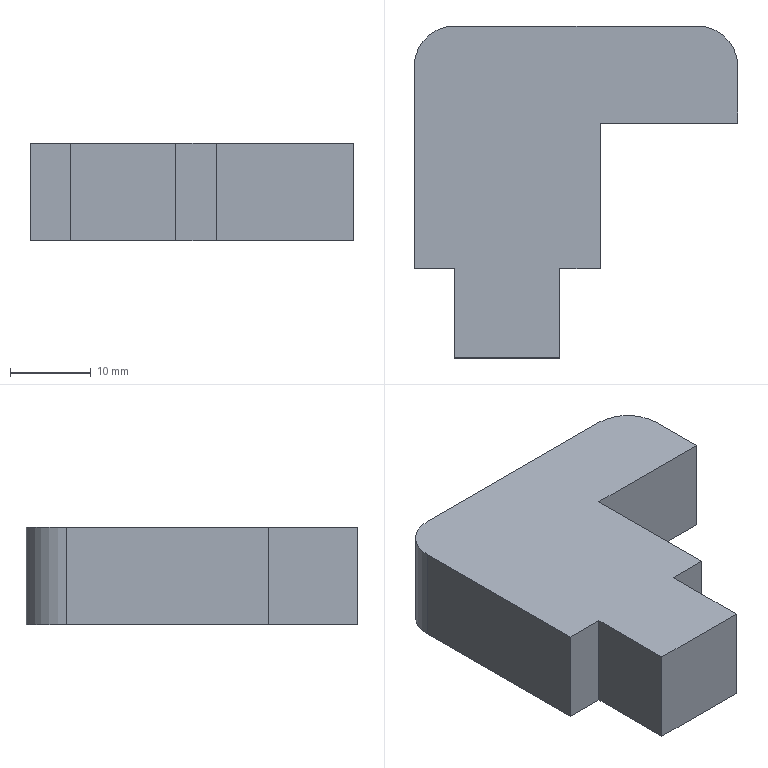Part | SolidWorks | features Fillet 1, FlatPattern 1, SMBaseFlange 1, SheetMetal 1 | 1 solid | 14 faces | box 40 x 41 x 12 mm | volume 12315 mm3 | plane 12 | cylinder 2 | commonest cylinder face diameters 10 x2
STEP:
#1=CARTESIAN_POINT('',(-40.,-14.,0.));
#2=VERTEX_POINT('',#1);
#3=CARTESIAN_POINT('',(-35.,-14.,0.));
#4=VERTEX_POINT('',#3);
#5=CARTESIAN_POINT('',(-35.,-14.,0.));
#6=DIRECTION('',(1.,0.,0.));
#7=VECTOR('',#6,1000.);
#8=LINE('',#5,#7);
#9=EDGE_CURVE('',#2,#4,#8,.T.);
#10=ORIENTED_EDGE('',*,*,#9,.F.);
#11=CARTESIAN_POINT('',(-40.,-14.,-12.));
#12=VERTEX_POINT('',#11);
#13=CARTESIAN_POINT('',(-40.,-14.,-12.));
#14=DIRECTION('',(0.,0.,1.));
#15=VECTOR('',#14,1000.);
#16=LINE('',#13,#15);
#17=EDGE_CURVE('',#12,#2,#16,.T.);
#18=ORIENTED_EDGE('',*,*,#17,.F.);
#19=CARTESIAN_POINT('',(-35.,-14.,-12.));
#20=VERTEX_POINT('',#19);
#21=CARTESIAN_POINT('',(-35.,-14.,-12.));
#22=DIRECTION('',(1.,0.,0.));
#23=VECTOR('',#22,1000.);
#24=LINE('',#21,#23);
#25=EDGE_CURVE('',#12,#20,#24,.T.);
#26=ORIENTED_EDGE('',*,*,#25,.T.);
#27=CARTESIAN_POINT('',(-35.,-14.,-12.));
#28=DIRECTION('',(0.,0.,1.));
#29=VECTOR('',#28,1000.);
#30=LINE('',#27,#29);
#31=EDGE_CURVE('',#20,#4,#30,.T.);
#32=ORIENTED_EDGE('',*,*,#31,.T.);
#33=EDGE_LOOP('',(#10,#18,#26,#32));
#34=FACE_OUTER_BOUND('',#33,.T.);
#35=CARTESIAN_POINT('',(-35.,-14.,-12.));
#36=DIRECTION('',(0.,-1.,0.));
#37=DIRECTION('',(1.,0.,0.));
#38=AXIS2_PLACEMENT_3D('',#35,#36,#37);
#39=PLANE('',#38);
#40=ADVANCED_FACE('',(#34),#39,.T.);
#41=CARTESIAN_POINT('',(-40.,11.,0.));
#42=VERTEX_POINT('',#41);
#43=CARTESIAN_POINT('',(-40.,-14.,0.));
#44=DIRECTION('',(0.,-1.,0.));
#45=VECTOR('',#44,1000.);
#46=LINE('',#43,#45);
#47=EDGE_CURVE('',#42,#2,#46,.T.);
#48=ORIENTED_EDGE('',*,*,#47,.F.);
#49=CARTESIAN_POINT('',(-40.,11.,-12.));
#50=VERTEX_POINT('',#49);
#51=CARTESIAN_POINT('',(-40.,11.,-12.));
#52=DIRECTION('',(0.,0.,-1.));
#53=VECTOR('',#52,1000.);
#54=LINE('',#51,#53);
#55=EDGE_CURVE('',#42,#50,#54,.T.);
#56=ORIENTED_EDGE('',*,*,#55,.T.);
#57=CARTESIAN_POINT('',(-40.,-14.,-12.));
#58=DIRECTION('',(0.,-1.,0.));
#59=VECTOR('',#58,1000.);
#60=LINE('',#57,#59);
#61=EDGE_CURVE('',#50,#12,#60,.T.);
#62=ORIENTED_EDGE('',*,*,#61,.T.);
#63=ORIENTED_EDGE('',*,*,#17,.T.);
#64=EDGE_LOOP('',(#48,#56,#62,#63));
#65=FACE_OUTER_BOUND('',#64,.T.);
#66=CARTESIAN_POINT('',(-40.,-14.,-12.));
#67=DIRECTION('',(-1.,0.,0.));
#68=DIRECTION('',(0.,-1.,0.));
#69=AXIS2_PLACEMENT_3D('',#66,#67,#68);
#70=PLANE('',#69);
#71=ADVANCED_FACE('',(#65),#70,.T.);
#72=CARTESIAN_POINT('',(-5.,16.,0.));
#73=VERTEX_POINT('',#72);
#74=CARTESIAN_POINT('',(-35.,16.,0.));
#75=VERTEX_POINT('',#74);
#76=CARTESIAN_POINT('',(-40.,16.,0.));
#77=DIRECTION('',(-1.,0.,0.));
#78=VECTOR('',#77,1000.);
#79=LINE('',#76,#78);
#80=EDGE_CURVE('',#73,#75,#79,.T.);
#81=ORIENTED_EDGE('',*,*,#80,.F.);
#82=CARTESIAN_POINT('',(-5.,16.,-12.));
#83=VERTEX_POINT('',#82);
#84=CARTESIAN_POINT('',(-5.,16.,-12.));
#85=DIRECTION('',(0.,0.,-1.));
#86=VECTOR('',#85,1000.);
#87=LINE('',#84,#86);
#88=EDGE_CURVE('',#73,#83,#87,.T.);
#89=ORIENTED_EDGE('',*,*,#88,.T.);
#90=CARTESIAN_POINT('',(-35.,16.,-12.));
#91=VERTEX_POINT('',#90);
#92=CARTESIAN_POINT('',(-40.,16.,-12.));
#93=DIRECTION('',(-1.,0.,0.));
#94=VECTOR('',#93,1000.);
#95=LINE('',#92,#94);
#96=EDGE_CURVE('',#83,#91,#95,.T.);
#97=ORIENTED_EDGE('',*,*,#96,.T.);
#98=CARTESIAN_POINT('',(-35.,16.,-12.));
#99=DIRECTION('',(0.,0.,1.));
#100=VECTOR('',#99,1000.);
#101=LINE('',#98,#100);
#102=EDGE_CURVE('',#91,#75,#101,.T.);
#103=ORIENTED_EDGE('',*,*,#102,.T.);
#104=EDGE_LOOP('',(#81,#89,#97,#103));
#105=FACE_OUTER_BOUND('',#104,.T.);
#106=CARTESIAN_POINT('',(-40.,16.,-12.));
#107=DIRECTION('',(0.,1.,0.));
#108=DIRECTION('',(0.,0.,1.));
#109=AXIS2_PLACEMENT_3D('',#106,#107,#108);
#110=PLANE('',#109);
#111=ADVANCED_FACE('',(#105),#110,.T.);
#112=CARTESIAN_POINT('',(0.,4.,-12.));
#113=VERTEX_POINT('',#112);
#114=CARTESIAN_POINT('',(0.,11.,-12.));
#115=VERTEX_POINT('',#114);
#116=CARTESIAN_POINT('',(0.,16.,-12.));
#117=DIRECTION('',(0.,1.,0.));
#118=VECTOR('',#117,1000.);
#119=LINE('',#116,#118);
#120=EDGE_CURVE('',#113,#115,#119,.T.);
#121=ORIENTED_EDGE('',*,*,#120,.T.);
#122=CARTESIAN_POINT('',(0.,11.,0.));
#123=VERTEX_POINT('',#122);
#124=CARTESIAN_POINT('',(0.,11.,-12.));
#125=DIRECTION('',(0.,0.,1.));
#126=VECTOR('',#125,1000.);
#127=LINE('',#124,#126);
#128=EDGE_CURVE('',#115,#123,#127,.T.);
#129=ORIENTED_EDGE('',*,*,#128,.T.);
#130=CARTESIAN_POINT('',(0.,4.,0.));
#131=VERTEX_POINT('',#130);
#132=CARTESIAN_POINT('',(0.,16.,0.));
#133=DIRECTION('',(0.,1.,0.));
#134=VECTOR('',#133,1000.);
#135=LINE('',#132,#134);
#136=EDGE_CURVE('',#131,#123,#135,.T.);
#137=ORIENTED_EDGE('',*,*,#136,.F.);
#138=CARTESIAN_POINT('',(0.,4.,-12.));
#139=DIRECTION('',(0.,0.,1.));
#140=VECTOR('',#139,1000.);
#141=LINE('',#138,#140);
#142=EDGE_CURVE('',#113,#131,#141,.T.);
#143=ORIENTED_EDGE('',*,*,#142,.F.);
#144=EDGE_LOOP('',(#121,#129,#137,#143));
#145=FACE_OUTER_BOUND('',#144,.T.);
#146=CARTESIAN_POINT('',(0.,16.,-12.));
#147=DIRECTION('',(1.,0.,0.));
#148=DIRECTION('',(0.,1.,0.));
#149=AXIS2_PLACEMENT_3D('',#146,#147,#148);
#150=PLANE('',#149);
#151=ADVANCED_FACE('',(#145),#150,.T.);
#152=CARTESIAN_POINT('',(-17.,4.,0.));
#153=VERTEX_POINT('',#152);
#154=CARTESIAN_POINT('',(0.,4.,0.));
#155=DIRECTION('',(1.,0.,0.));
#156=VECTOR('',#155,1000.);
#157=LINE('',#154,#156);
#158=EDGE_CURVE('',#153,#131,#157,.T.);
#159=ORIENTED_EDGE('',*,*,#158,.F.);
#160=CARTESIAN_POINT('',(-17.,4.,-12.));
#161=VERTEX_POINT('',#160);
#162=CARTESIAN_POINT('',(-17.,4.,-12.));
#163=DIRECTION('',(0.,0.,1.));
#164=VECTOR('',#163,1000.);
#165=LINE('',#162,#164);
#166=EDGE_CURVE('',#161,#153,#165,.T.);
#167=ORIENTED_EDGE('',*,*,#166,.F.);
#168=CARTESIAN_POINT('',(0.,4.,-12.));
#169=DIRECTION('',(1.,0.,0.));
#170=VECTOR('',#169,1000.);
#171=LINE('',#168,#170);
#172=EDGE_CURVE('',#161,#113,#171,.T.);
#173=ORIENTED_EDGE('',*,*,#172,.T.);
#174=ORIENTED_EDGE('',*,*,#142,.T.);
#175=EDGE_LOOP('',(#159,#167,#173,#174));
#176=FACE_OUTER_BOUND('',#175,.T.);
#177=CARTESIAN_POINT('',(0.,4.,-12.));
#178=DIRECTION('',(0.,-1.,0.));
#179=DIRECTION('',(1.,0.,0.));
#180=AXIS2_PLACEMENT_3D('',#177,#178,#179);
#181=PLANE('',#180);
#182=ADVANCED_FACE('',(#176),#181,.T.);
#183=CARTESIAN_POINT('',(-17.,-14.,0.));
#184=VERTEX_POINT('',#183);
#185=CARTESIAN_POINT('',(-17.,4.,0.));
#186=DIRECTION('',(0.,1.,0.));
#187=VECTOR('',#186,1000.);
#188=LINE('',#185,#187);
#189=EDGE_CURVE('',#184,#153,#188,.T.);
#190=ORIENTED_EDGE('',*,*,#189,.F.);
#191=CARTESIAN_POINT('',(-17.,-14.,-12.));
#192=VERTEX_POINT('',#191);
#193=CARTESIAN_POINT('',(-17.,-14.,-12.));
#194=DIRECTION('',(0.,0.,1.));
#195=VECTOR('',#194,1000.);
#196=LINE('',#193,#195);
#197=EDGE_CURVE('',#192,#184,#196,.T.);
#198=ORIENTED_EDGE('',*,*,#197,.F.);
#199=CARTESIAN_POINT('',(-17.,4.,-12.));
#200=DIRECTION('',(0.,1.,0.));
#201=VECTOR('',#200,1000.);
#202=LINE('',#199,#201);
#203=EDGE_CURVE('',#192,#161,#202,.T.);
#204=ORIENTED_EDGE('',*,*,#203,.T.);
#205=ORIENTED_EDGE('',*,*,#166,.T.);
#206=EDGE_LOOP('',(#190,#198,#204,#205));
#207=FACE_OUTER_BOUND('',#206,.T.);
#208=CARTESIAN_POINT('',(-17.,4.,-12.));
#209=DIRECTION('',(1.,0.,0.));
#210=DIRECTION('',(0.,1.,0.));
#211=AXIS2_PLACEMENT_3D('',#208,#209,#210);
#212=PLANE('',#211);
#213=ADVANCED_FACE('',(#207),#212,.T.);
#214=CARTESIAN_POINT('',(-22.,-14.,0.));
#215=VERTEX_POINT('',#214);
#216=CARTESIAN_POINT('',(-17.,-14.,0.));
#217=DIRECTION('',(1.,0.,0.));
#218=VECTOR('',#217,1000.);
#219=LINE('',#216,#218);
#220=EDGE_CURVE('',#215,#184,#219,.T.);
#221=ORIENTED_EDGE('',*,*,#220,.F.);
#222=CARTESIAN_POINT('',(-22.,-14.,-12.));
#223=VERTEX_POINT('',#222);
#224=CARTESIAN_POINT('',(-22.,-14.,-12.));
#225=DIRECTION('',(0.,0.,1.));
#226=VECTOR('',#225,1000.);
#227=LINE('',#224,#226);
#228=EDGE_CURVE('',#223,#215,#227,.T.);
#229=ORIENTED_EDGE('',*,*,#228,.F.);
#230=CARTESIAN_POINT('',(-17.,-14.,-12.));
#231=DIRECTION('',(1.,0.,0.));
#232=VECTOR('',#231,1000.);
#233=LINE('',#230,#232);
#234=EDGE_CURVE('',#223,#192,#233,.T.);
#235=ORIENTED_EDGE('',*,*,#234,.T.);
#236=ORIENTED_EDGE('',*,*,#197,.T.);
#237=EDGE_LOOP('',(#221,#229,#235,#236));
#238=FACE_OUTER_BOUND('',#237,.T.);
#239=CARTESIAN_POINT('',(-17.,-14.,-12.));
#240=DIRECTION('',(0.,-1.,0.));
#241=DIRECTION('',(0.,0.,-1.));
#242=AXIS2_PLACEMENT_3D('',#239,#240,#241);
#243=PLANE('',#242);
#244=ADVANCED_FACE('',(#238),#243,.T.);
#245=CARTESIAN_POINT('',(-22.,-25.,0.));
#246=VERTEX_POINT('',#245);
#247=CARTESIAN_POINT('',(-22.,-25.,0.));
#248=DIRECTION('',(0.,1.,0.));
#249=VECTOR('',#248,1000.);
#250=LINE('',#247,#249);
#251=EDGE_CURVE('',#246,#215,#250,.T.);
#252=ORIENTED_EDGE('',*,*,#251,.F.);
#253=CARTESIAN_POINT('',(-22.,-25.,-12.));
#254=VERTEX_POINT('',#253);
#255=CARTESIAN_POINT('',(-22.,-25.,-12.));
#256=DIRECTION('',(0.,0.,1.));
#257=VECTOR('',#256,1000.);
#258=LINE('',#255,#257);
#259=EDGE_CURVE('',#254,#246,#258,.T.);
#260=ORIENTED_EDGE('',*,*,#259,.F.);
#261=CARTESIAN_POINT('',(-22.,-25.,-12.));
#262=DIRECTION('',(0.,1.,0.));
#263=VECTOR('',#262,1000.);
#264=LINE('',#261,#263);
#265=EDGE_CURVE('',#254,#223,#264,.T.);
#266=ORIENTED_EDGE('',*,*,#265,.T.);
#267=ORIENTED_EDGE('',*,*,#228,.T.);
#268=EDGE_LOOP('',(#252,#260,#266,#267));
#269=FACE_OUTER_BOUND('',#268,.T.);
#270=CARTESIAN_POINT('',(-22.,-25.,-12.));
#271=DIRECTION('',(1.,0.,0.));
#272=DIRECTION('',(0.,0.,-1.));
#273=AXIS2_PLACEMENT_3D('',#270,#271,#272);
#274=PLANE('',#273);
#275=ADVANCED_FACE('',(#269),#274,.T.);
#276=CARTESIAN_POINT('',(-35.,-25.,0.));
#277=VERTEX_POINT('',#276);
#278=CARTESIAN_POINT('',(-35.,-25.,0.));
#279=DIRECTION('',(1.,0.,0.));
#280=VECTOR('',#279,1000.);
#281=LINE('',#278,#280);
#282=EDGE_CURVE('',#277,#246,#281,.T.);
#283=ORIENTED_EDGE('',*,*,#282,.F.);
#284=CARTESIAN_POINT('',(-35.,-25.,-12.));
#285=VERTEX_POINT('',#284);
#286=CARTESIAN_POINT('',(-35.,-25.,-12.));
#287=DIRECTION('',(0.,0.,1.));
#288=VECTOR('',#287,1000.);
#289=LINE('',#286,#288);
#290=EDGE_CURVE('',#285,#277,#289,.T.);
#291=ORIENTED_EDGE('',*,*,#290,.F.);
#292=CARTESIAN_POINT('',(-35.,-25.,-12.));
#293=DIRECTION('',(1.,0.,0.));
#294=VECTOR('',#293,1000.);
#295=LINE('',#292,#294);
#296=EDGE_CURVE('',#285,#254,#295,.T.);
#297=ORIENTED_EDGE('',*,*,#296,.T.);
#298=ORIENTED_EDGE('',*,*,#259,.T.);
#299=EDGE_LOOP('',(#283,#291,#297,#298));
#300=FACE_OUTER_BOUND('',#299,.T.);
#301=CARTESIAN_POINT('',(-35.,-25.,-12.));
#302=DIRECTION('',(0.,-1.,0.));
#303=DIRECTION('',(0.,0.,-1.));
#304=AXIS2_PLACEMENT_3D('',#301,#302,#303);
#305=PLANE('',#304);
#306=ADVANCED_FACE('',(#300),#305,.T.);
#307=CARTESIAN_POINT('',(-35.,-14.,0.));
#308=DIRECTION('',(0.,-1.,0.));
#309=VECTOR('',#308,1000.);
#310=LINE('',#307,#309);
#311=EDGE_CURVE('',#4,#277,#310,.T.);
#312=ORIENTED_EDGE('',*,*,#311,.F.);
#313=ORIENTED_EDGE('',*,*,#31,.F.);
#314=CARTESIAN_POINT('',(-35.,-14.,-12.));
#315=DIRECTION('',(0.,-1.,0.));
#316=VECTOR('',#315,1000.);
#317=LINE('',#314,#316);
#318=EDGE_CURVE('',#20,#285,#317,.T.);
#319=ORIENTED_EDGE('',*,*,#318,.T.);
#320=ORIENTED_EDGE('',*,*,#290,.T.);
#321=EDGE_LOOP('',(#312,#313,#319,#320));
#322=FACE_OUTER_BOUND('',#321,.T.);
#323=CARTESIAN_POINT('',(-35.,-14.,-12.));
#324=DIRECTION('',(-1.,0.,0.));
#325=DIRECTION('',(0.,-1.,0.));
#326=AXIS2_PLACEMENT_3D('',#323,#324,#325);
#327=PLANE('',#326);
#328=ADVANCED_FACE('',(#322),#327,.T.);
#329=ORIENTED_EDGE('',*,*,#96,.F.);
#330=CARTESIAN_POINT('',(-5.,11.,-12.));
#331=DIRECTION('',(0.,0.,-1.));
#332=DIRECTION('',(-1.,0.,0.));
#333=AXIS2_PLACEMENT_3D('',#330,#331,#332);
#334=CIRCLE('',#333,5.);
#335=EDGE_CURVE('',#83,#115,#334,.T.);
#336=ORIENTED_EDGE('',*,*,#335,.T.);
#337=ORIENTED_EDGE('',*,*,#120,.F.);
#338=ORIENTED_EDGE('',*,*,#172,.F.);
#339=ORIENTED_EDGE('',*,*,#203,.F.);
#340=ORIENTED_EDGE('',*,*,#234,.F.);
#341=ORIENTED_EDGE('',*,*,#265,.F.);
#342=ORIENTED_EDGE('',*,*,#296,.F.);
#343=ORIENTED_EDGE('',*,*,#318,.F.);
#344=ORIENTED_EDGE('',*,*,#25,.F.);
#345=ORIENTED_EDGE('',*,*,#61,.F.);
#346=CARTESIAN_POINT('',(-35.,11.,-12.));
#347=DIRECTION('',(0.,0.,-1.));
#348=DIRECTION('',(-1.,0.,0.));
#349=AXIS2_PLACEMENT_3D('',#346,#347,#348);
#350=CIRCLE('',#349,5.);
#351=EDGE_CURVE('',#50,#91,#350,.T.);
#352=ORIENTED_EDGE('',*,*,#351,.T.);
#353=EDGE_LOOP('',(#329,#336,#337,#338,#339,#340,#341,#342,#343,#344,#345,#352));
#354=FACE_OUTER_BOUND('',#353,.T.);
#355=CARTESIAN_POINT('',(0.,0.,-12.));
#356=DIRECTION('',(0.,0.,-1.));
#357=DIRECTION('',(-1.,0.,0.));
#358=AXIS2_PLACEMENT_3D('',#355,#356,#357);
#359=PLANE('',#358);
#360=ADVANCED_FACE('',(#354),#359,.T.);
#361=ORIENTED_EDGE('',*,*,#136,.T.);
#362=CARTESIAN_POINT('',(-5.,11.,0.));
#363=DIRECTION('',(0.,0.,1.));
#364=DIRECTION('',(-1.,0.,0.));
#365=AXIS2_PLACEMENT_3D('',#362,#363,#364);
#366=CIRCLE('',#365,5.);
#367=EDGE_CURVE('',#123,#73,#366,.T.);
#368=ORIENTED_EDGE('',*,*,#367,.T.);
#369=ORIENTED_EDGE('',*,*,#80,.T.);
#370=CARTESIAN_POINT('',(-35.,11.,0.));
#371=DIRECTION('',(0.,0.,1.));
#372=DIRECTION('',(-1.,0.,0.));
#373=AXIS2_PLACEMENT_3D('',#370,#371,#372);
#374=CIRCLE('',#373,5.);
#375=EDGE_CURVE('',#75,#42,#374,.T.);
#376=ORIENTED_EDGE('',*,*,#375,.T.);
#377=ORIENTED_EDGE('',*,*,#47,.T.);
#378=ORIENTED_EDGE('',*,*,#9,.T.);
#379=ORIENTED_EDGE('',*,*,#311,.T.);
#380=ORIENTED_EDGE('',*,*,#282,.T.);
#381=ORIENTED_EDGE('',*,*,#251,.T.);
#382=ORIENTED_EDGE('',*,*,#220,.T.);
#383=ORIENTED_EDGE('',*,*,#189,.T.);
#384=ORIENTED_EDGE('',*,*,#158,.T.);
#385=EDGE_LOOP('',(#361,#368,#369,#376,#377,#378,#379,#380,#381,#382,#383,#384));
#386=FACE_OUTER_BOUND('',#385,.T.);
#387=CARTESIAN_POINT('',(0.,0.,0.));
#388=DIRECTION('',(0.,0.,-1.));
#389=DIRECTION('',(-1.,0.,0.));
#390=AXIS2_PLACEMENT_3D('',#387,#388,#389);
#391=PLANE('',#390);
#392=ADVANCED_FACE('',(#386),#391,.F.);
#393=ORIENTED_EDGE('',*,*,#335,.F.);
#394=ORIENTED_EDGE('',*,*,#88,.F.);
#395=ORIENTED_EDGE('',*,*,#367,.F.);
#396=ORIENTED_EDGE('',*,*,#128,.F.);
#397=EDGE_LOOP('',(#393,#394,#395,#396));
#398=FACE_OUTER_BOUND('',#397,.T.);
#399=CARTESIAN_POINT('',(-5.,11.,-12.));
#400=DIRECTION('',(0.,0.,1.));
#401=DIRECTION('',(1.,0.,0.));
#402=AXIS2_PLACEMENT_3D('',#399,#400,#401);
#403=CYLINDRICAL_SURFACE('',#402,5.);
#404=ADVANCED_FACE('',(#398),#403,.T.);
#405=ORIENTED_EDGE('',*,*,#351,.F.);
#406=ORIENTED_EDGE('',*,*,#55,.F.);
#407=ORIENTED_EDGE('',*,*,#375,.F.);
#408=ORIENTED_EDGE('',*,*,#102,.F.);
#409=EDGE_LOOP('',(#405,#406,#407,#408));
#410=FACE_OUTER_BOUND('',#409,.T.);
#411=CARTESIAN_POINT('',(-35.,11.,-12.));
#412=DIRECTION('',(0.,0.,1.));
#413=DIRECTION('',(1.,0.,0.));
#414=AXIS2_PLACEMENT_3D('',#411,#412,#413);
#415=CYLINDRICAL_SURFACE('',#414,5.);
#416=ADVANCED_FACE('',(#410),#415,.T.);
#417=CLOSED_SHELL('',(#40,#71,#111,#151,#182,#213,#244,#275,#306,#328,#360,#392,#404,#416));
#418=MANIFOLD_SOLID_BREP('',#417);
#419=CARTESIAN_POINT('',(0.,0.,0.));
#420=DIRECTION('',(0.,0.,1.));
#421=DIRECTION('',(1.,0.,0.));
#422=AXIS2_PLACEMENT_3D('',#419,#420,#421);
#423=(LENGTH_UNIT()NAMED_UNIT(*)SI_UNIT(.MILLI.,.METRE.));
#424=UNCERTAINTY_MEASURE_WITH_UNIT(LENGTH_MEASURE(0.00001),#423,'','');
#425=(NAMED_UNIT(*)PLANE_ANGLE_UNIT()SI_UNIT($,.RADIAN.));
#426=(NAMED_UNIT(*)SI_UNIT($,.STERADIAN.)SOLID_ANGLE_UNIT());
#427=(GEOMETRIC_REPRESENTATION_CONTEXT(3)GLOBAL_UNCERTAINTY_ASSIGNED_CONTEXT((#424))GLOBAL_UNIT_ASSIGNED_CONTEXT((#423,#425,#426))REPRESENTATION_CONTEXT('',''));
#428=ADVANCED_BREP_SHAPE_REPRESENTATION('',(#418,#422),#427);